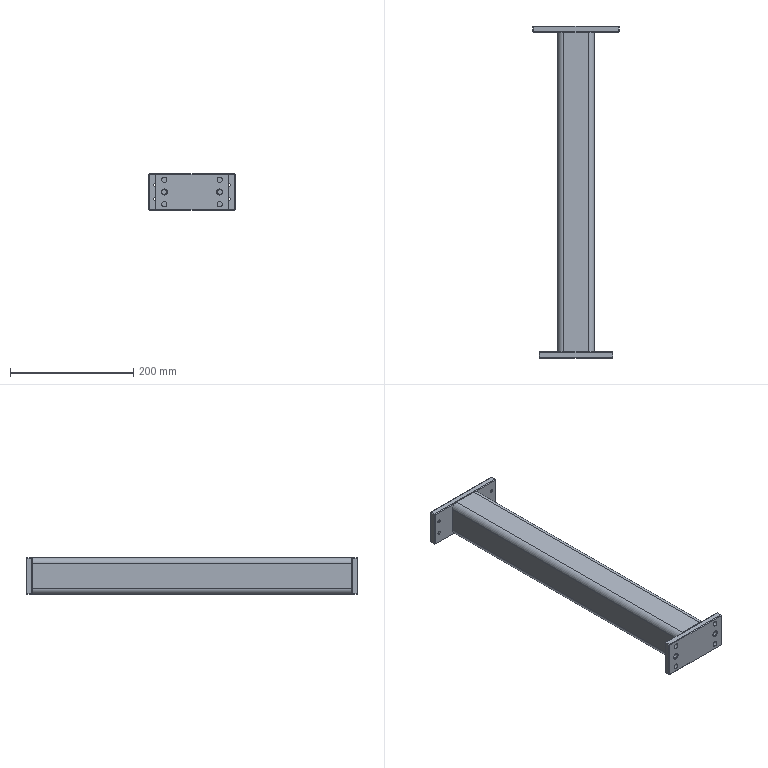Part | SolidWorks | features Chamfer 3, ICE 3, HoleWzd 2, 3DProfileFeature 1, WeldMemberFeat 1, WeldmentFeature 1 | 3 solids | 98 faces | box 140 x 539 x 60 mm | volume 688528 mm3 | plane 62 | cylinder 28 | cone 8 | commonest cylinder face diameters 5 x8 8.6 x8 8 x4 10 x4 20 x4